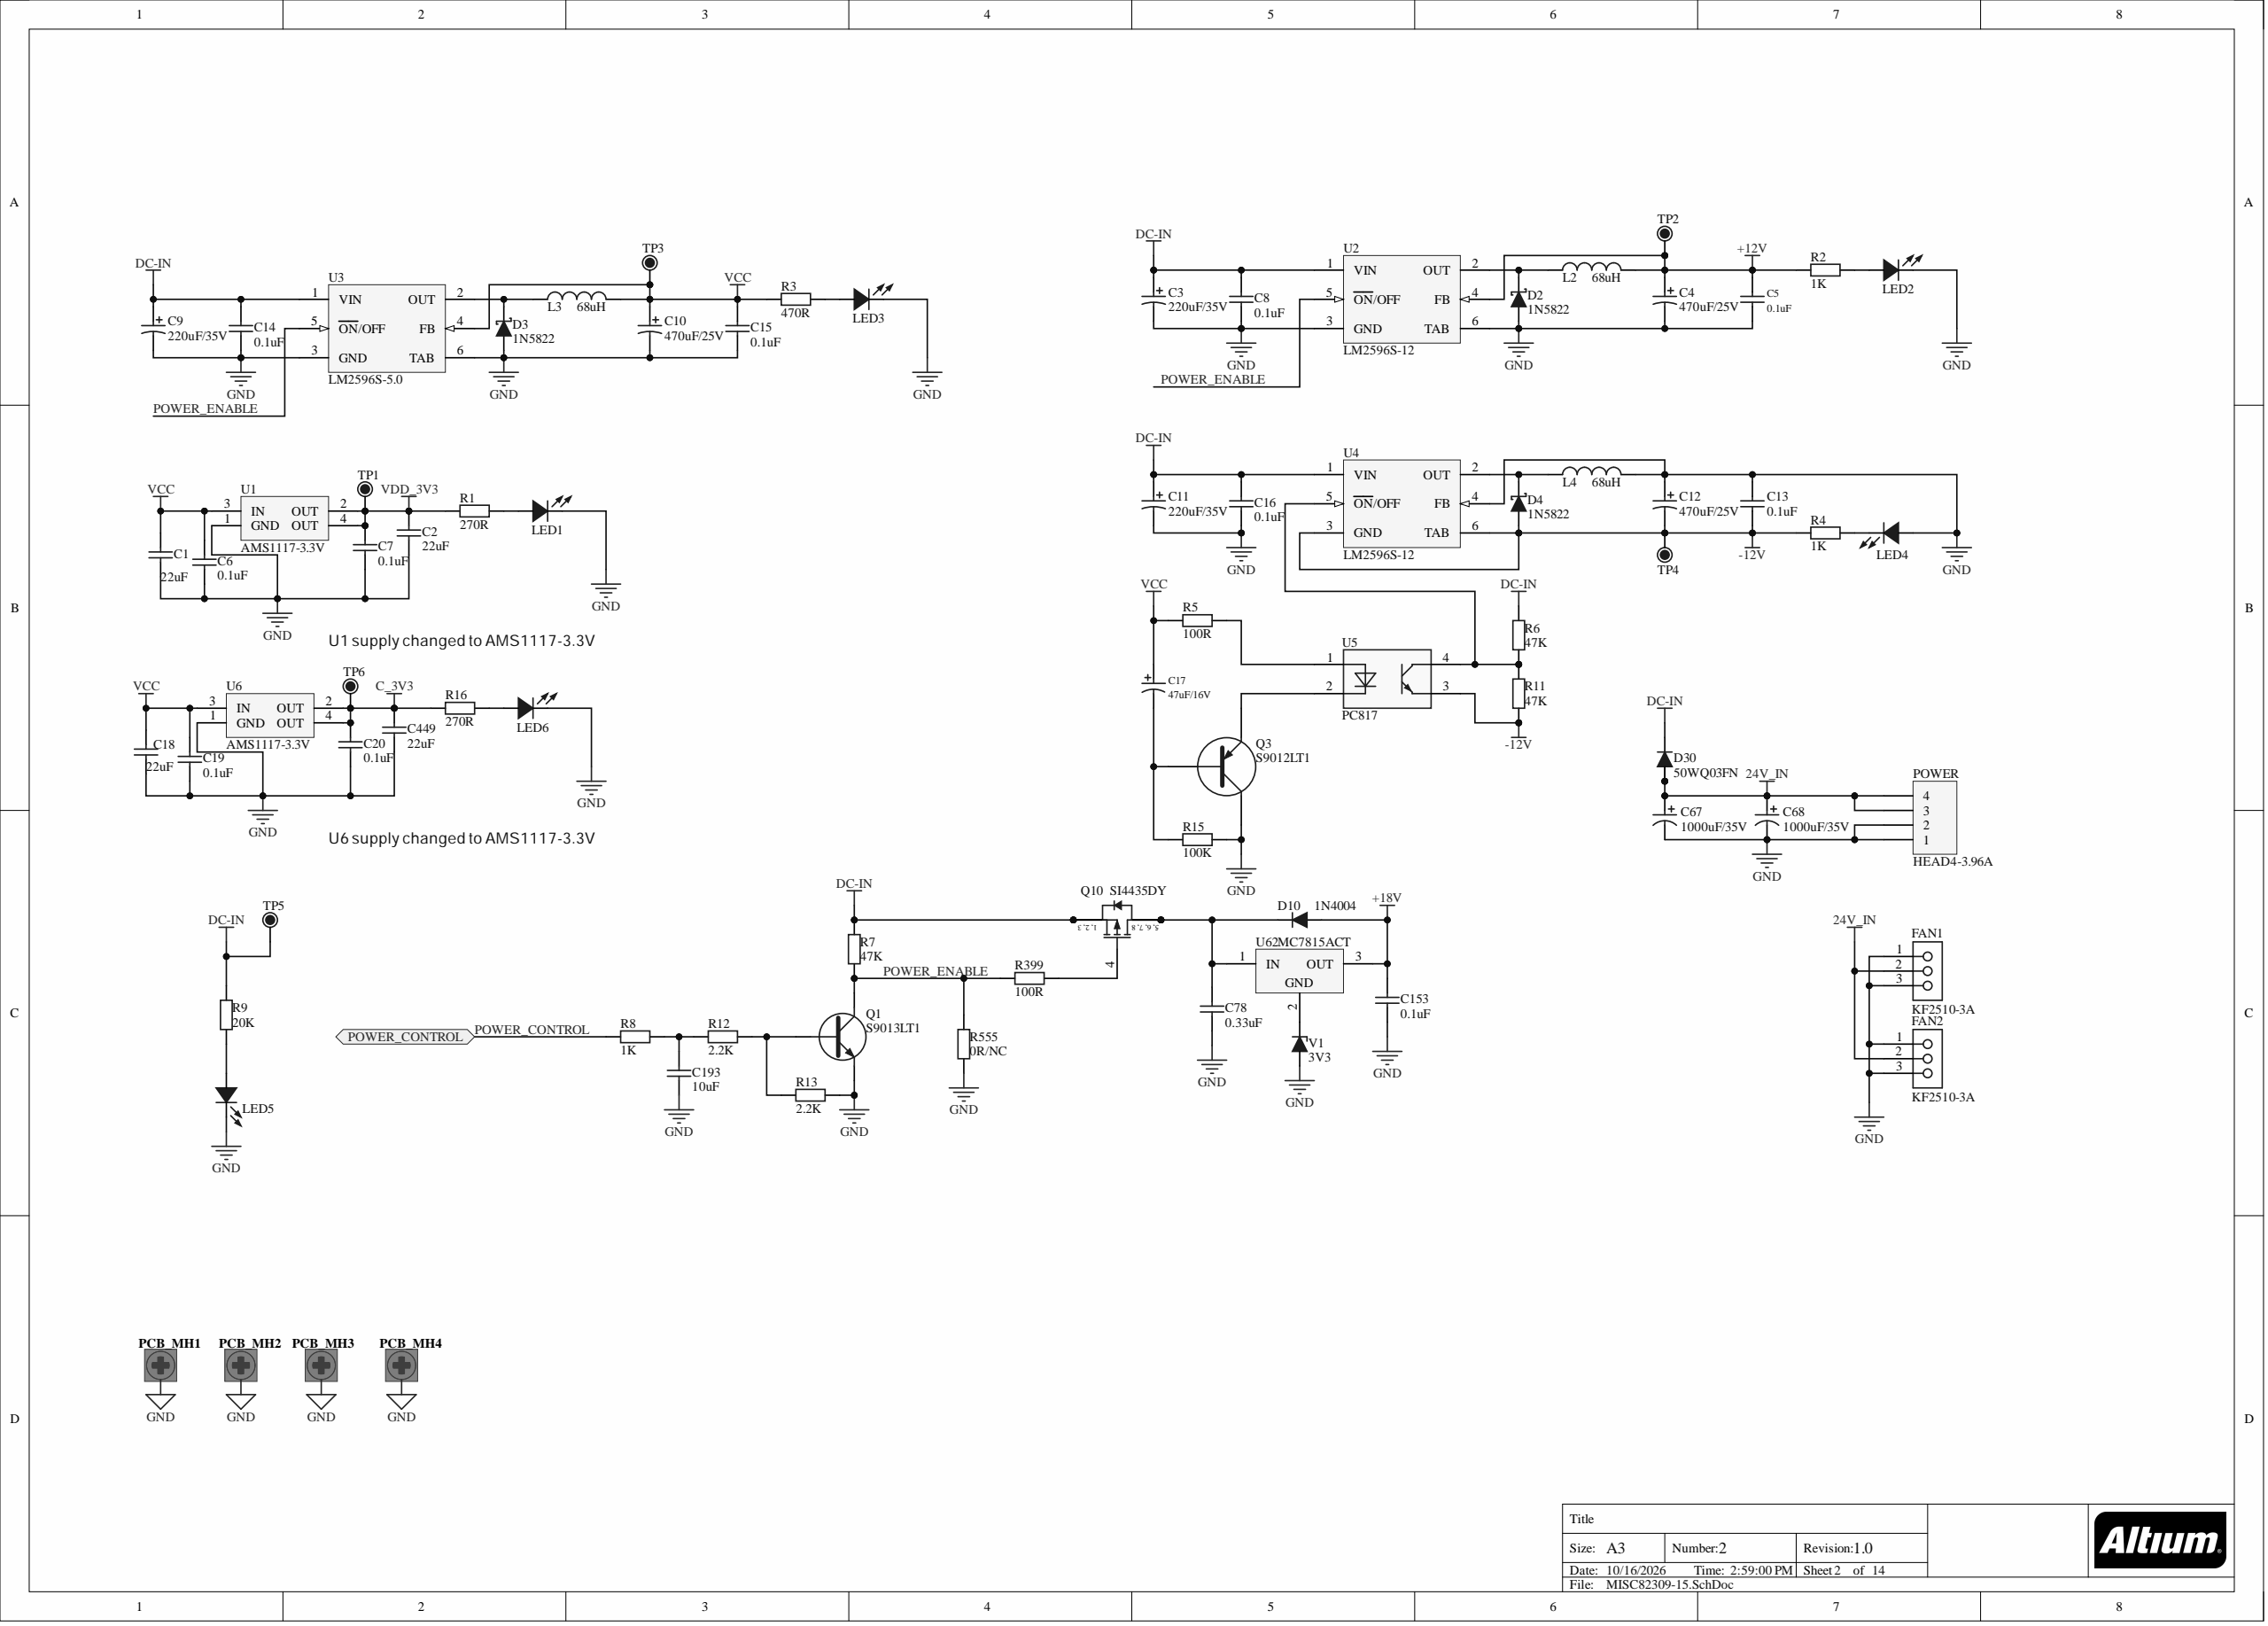Circuit board | Altium Designer | 747 parts | 576 nets | one sheet of the schematic
Parts on this sheet (reference | value | footprint):
C1 | 22uF | C0805
C2 | 22uF | C0805
C3 | 220uF/35V | E8X10,2
C4 | 470uF/25V | E10X10.2
C5 | 0.1uF | C1206
C6 | 0.1uF | C0603
C7 | 0.1uF | C0603
C8 | 0.1uF | C1206
C9 | 220uF/35V | E8X10,2
C10 | 470uF/25V | E10X10.2
C11 | 220uF/35V | E8X10,2
C12 | 470uF/25V | E10X10.2
C13 | 0.1uF | C1206
C14 | 0.1uF | C1206
C15 | 0.1uF | C1206
C16 | 0.1uF | C1206
C17 | 47uF/16V | E5X5.4
C18 | 22uF | C0805
C19 | 0.1uF | C0603
C20 | 0.1uF | C0603
C67 | 1000uF/35V | CAP-EL-12x20
C68 | 1000uF/35V | CAP-EL-12x20
C78 | 0.33uF | C1206
C153 | 0.1uF | C1206
C193 | 10uF | C0805
C449 | 22uF | C0805
D2 | 1N5822 | D1810
D3 | 1N5822 | D1810
D4 | 1N5822 | D1810
D10 | 1N4004 | DO-41 - 10.46mm
D30 | 50WQ03FN | TO-252AA
FAN1 | KF2510-3A | KF2510-3A
FAN2 | KF2510-3A | KF2510-3A
L2 | 68uH | L330
L3 | 68uH | L330
L4 | 68uH | L330
LED1 | LED | LED_0805
LED2 | LED | LED_0805
LED3 | LED | LED_0805
LED4 | LED | LED_0805
LED5 | LED | LED_0805
LED6 | LED | LED_0805
PCB_MH1
PCB_MH2
PCB_MH3
PCB_MH4
POWER | HEAD4-3.96A | VH-3_96-4
Q1 | S9013LT1 | SOT-23
Q3 | S9012LT1 | SOT-23
Q10 | SI4435DY | SO-8_N
R1 | 270R | RES_0805
R2 | 1K | RES_0805
R3 | 470R | RES_0805
R4 | 1K | RES_0805
R5 | 100R | RES_0805
R6 | 47K | RES_0805
R7 | 47K | RES_0805
R8 | 1K | RES_0805
R9 | 20K | RES_0805
R11 | 47K | RES_0805
R12 | 2.2K | RES_0805
R13 | 2.2K | RES_0805
R15 | 100K | RES_0805
R16 | 270R | RES_0805
R399 | 100R | RES_0805
R555 | 0R/NC | RES_0603
TP1 | TP | TPOINT
TP2 | TP | TPOINT
TP3 | TP | TPOINT
TP4 | TP | TPOINT
TP5 | TP | TPOINT
TP6 | TP | TPOINT
U1 | AMS1117-3.3V | SOT223
U2 | LM2596S-12 | TS5B_N
U3 | LM2596S-5.0 | TS5B_N
U4 | LM2596S-12 | TS5B_N
U5 | PC817 | SOIC_4N
U6 | AMS1117-3.3V | SOT223
V1 | 3V3 | DO-213AA
Nets of these parts (net: part-pin ...):
VDD_3V3: C2-2 C7-2 R1-1 TP1-1 U1-2 U1-4
VCC: C1-2 C6-2 C10-1 C15-1 C17-1 C18-2 C19-2 L3-2 R3-1 R5-1 TP3-1 U1-3 U3-4 U6-3
POWER_ENABLE: Q1-3 R7-1 R399-2 R555-2 U2-5 U3-5
POWER_CONTROL: R8-1
NetU62_2: V1-2
NetR6_1: R6-1 R11-2 U4-5 U5-4
NetR5_2: R5-2 U5-1
NetQ10_4: Q10-4 R399-1
NetQ3_2: Q3-2 U5-2
NetQ1_1: Q1-1 R12-2 R13-1
NetLED6_1: LED6-1 R16-2
NetLED5_1: LED5-1 R9-1
NetLED4_2: LED4-2 R4-2
NetLED3_1: LED3-1 R3-2
NetLED2_1: LED2-1 R2-2
NetLED1_1: LED1-1 R1-2
NetD4_2: D4-2 L4-1 U4-2
NetD3_2: D3-2 L3-1 U3-2
NetD2_2: D2-2 L2-1 U2-2
NetC193_2: C193-2 R8-2 R12-1
NetC78_1: C78-1 D10-2 Q10-5 Q10-6 Q10-7 Q10-8
NetC17_2: C17-2 Q3-1 R15-1
GND: C1-1 C2-1 C3-2 C4-2 C5-2 C6-1 C7-1 C8-1 C9-2 C10-2 C11-2 C12-1 C13-1 C14-1 C15-2 C16-1 C18-1 C19-1 C20-1 C67-2 C68-2 C78-2 C153-2 C193-1 C449-1 D2-1 D3-1 FAN1-1 FAN1-3 FAN2-1 FAN2-3 L4-2 LED1-2 LED2-2 LED3-2 LED4-1 LED5-2 LED6-2 POWER-1 POWER-2 Q1-2 Q3-3 R13-2 R15-2 R555-1 U1-1 U2-3 U2-6 U3-3 U3-6 U4-4 U6-1 V1-1
DC-IN: C3-1 C8-2 C9-1 C11-1 C14-2 C16-2 D30-4 Q10-1 Q10-2 Q10-3 R6-2 R7-2 R9-2 TP5-1 U2-1 U3-1 U4-1
C_3V3: C20-2 C449-2 R16-1 TP6-1 U6-2 U6-4
-12V: C12-2 C13-2 D4-1 R4-1 R11-1 TP4-1 U4-3 U4-6 U5-3
+18V: C153-1 D10-1
+12V: C4-1 C5-1 L2-2 R2-1 TP2-1 U2-4
24V_IN: C67-1 C68-1 D30-1 D30-3 FAN1-2 FAN2-2 POWER-3 POWER-4